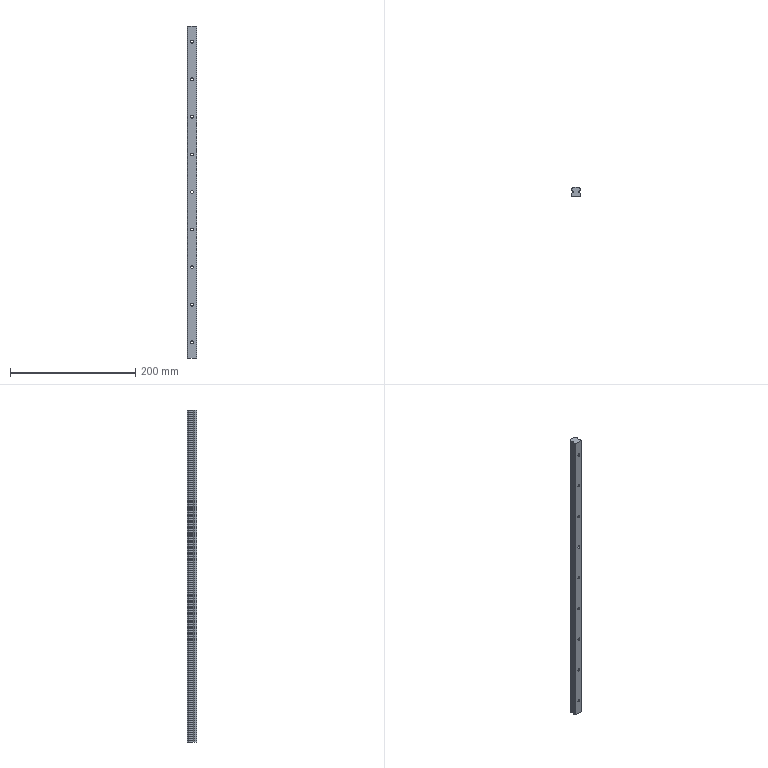Part | STEP file | ASND-0110-HGR15_1TCTF01sb | 1 solid | 81 faces | box 15 x 15 x 530 mm | volume 97544 mm3 | cylinder 50 | plane 31 | commonest cylinder face diameters 4.5 x18 8 x12 0.8 x8 7.5 x6 3.24 x4 2 x2